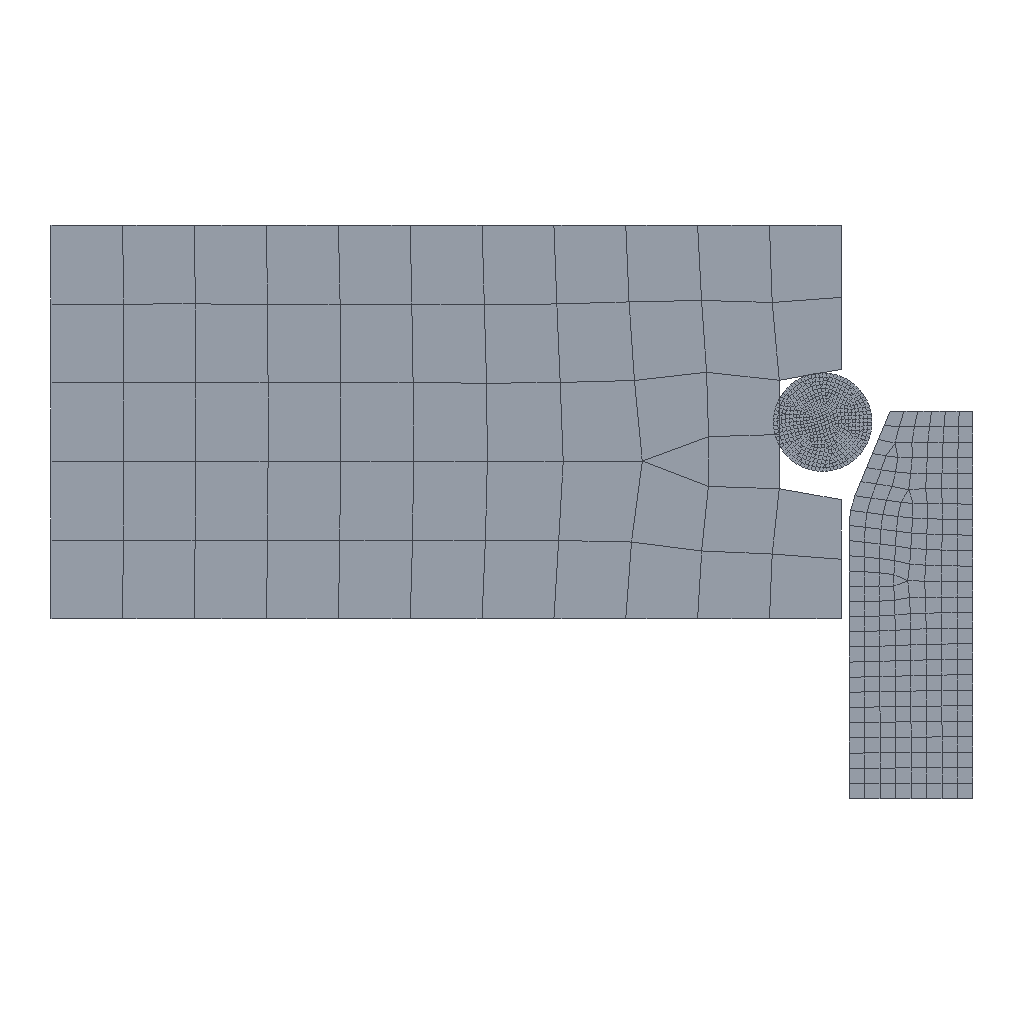Simulation study | ansys workbench
Set-up summary:
category,name,step,type,value,unit,region
solver,ansys_workbench
units,mm-N-s-tonne (MPa),,stated,"/units,MPA"
analysis,LS1,,static
load_step,LS1,LS1,static,nsubst=5; time=1
load_step,LS2,LS2,static,nsubst=100; time=2
mesh,nodes,,,2717
mesh,elements,,,1054
element_type,PLANE183,,,858
element_type,CONTA172,,,196
material,oxingquan,,behaviors,"hyperelastic; tb hype,NEO"
material,Structural Steel,,E,200000,tonne s^-2 mm^-1
material,Structural Steel,,nu,0.3
material,Structural Steel,,density,7.85e-09,tonne mm^-3
material,Structural Steel,,conductivity,60.5,tonne mm s^-3 C^-1
material,Structural Steel,,specific_heat,4.34e+08,mm^2 s^-2 C^-1
material,Structural Steel,,cte,1.2e-05,C^-1
material,Structural Steel,,permeability,10000
material,Structural Steel,,resistivity,0.00017,ohm mm
bc,Fixed Supports,model,fixed,[dofs=ALL],,_FIXEDSU
bc,Constant Zero Displacement X,model,fixed,[dofs=UX],,_DISPZEROUX
bc,Set Displacements,LS1,prescribed uy,10 [dofs=UY],,_CM54UY_YP
contact,Frictional - O ring To Surface Body,,standard (frictionless/frictional),friction=0.2; element=CONTA172
contact,Frictional - O ring To bar,,standard (frictionless/frictional),friction=0.2; element=CONTA172
named_set,_FIXEDSU,,node,23
named_set,_DISPZEROUX,,node,17
named_set,_CM54UY_YP,,node,17
Ansys APDL input file, long lists of numbers shortened:
/batch
/config,noeldb,1     ! force off writing results to database
*get,_wallstrt,active,,time,wall
! ANSYS input file written by Workbench version 2025 R2
! File used for geometry attach:
/title,O_________--____ (A5)
! ****** Begin Custom Load Command Snippet ******
/COM, ACT Extensions:
/COM,     LSDYNA, 2025.2
/COM,/COM,     ANSYSMotion, 2025.2
/COM,
! ****** End   Custom Load Command Snippet ******
*DIM,_wb_ProjectScratch_dir,string,248
_wb_ProjectScratch_dir(1) = ''
/com,--- Data in consistent NMM units. See Solving Units in the help system for more information.
/units,MPA
/nopr
/wb,file,start              !  signify a WB generated input file
/prep7
! Turn off shape checking because checks already performed inside WB mesher.
! See help system for more information.
SHPP,OFF,,NOWARN
/nolist
etcon,set             ! allow ANSYS to choose best KEYOP's for 180x elements, resets any applicable keyopt to MAPDL defaults
/com,*********** Send User Defined Coordinate System(s) ***********
csys,0
/com,*********** Nodes for the whole assembly ***********
nblock,3,,2988
(1i9,3e20.9e3)
        1     4.845794036E+01    -2.341433940E+00     0.000000000E+00
! (2716 more lines like these left out)
-1
/wb,elem,start            !  set before creation of elements
/com,*********** Elements for Body 1 'O ring' ***********
et,1,183
keyo,1,3,1
MAT,1 $ TYPE,1 $ REAL,1 $ SECNUM,1 $ ESYS,0
eblock,11,COMPACT,,605
(11i9)
       80       45       59      554      554      696     1375      554     1382
! (604 more lines like these left out)
-1
secnum,1    ! reset the section ID to default
/com,*********** Elements for Body 2 'Surface Body' ***********
et,2,183
keyo,2,3,1
MAT,2 $ TYPE,2 $ REAL,2 $ SECNUM,2 $ ESYS,0
eblock,11,COMPACT,,56
(11i9)
      650     1926     1927     1914     1914     2045     2046     1914     2047
! (55 more lines like these left out)
-1
secnum,1    ! reset the section ID to default
/com,*********** Elements for Body 3 'bar' ***********
et,3,183
keyo,3,3,1
MAT,3 $ TYPE,3 $ REAL,3 $ SECNUM,3 $ ESYS,0
eblock,11,COMPACT,,197
(11i9)
      723     2201     2203     2204     2204     2555     2557     2204     2558
! (196 more lines like these left out)
-1
secnum,1    ! reset the section ID to default
/wb,elem,end               !  done creating elements
toffst,273.15,      ! Temperature offset from absolute zero
/com,*********** Set Reference Temperature ***********
tref,22.
/wb,mat,start              !  starting to send materials
/com,*********** Send Materials ***********
TB,HYPE,1,1,1,NEO
TBDATA,1,20,0.015
Temperature = 'TEMP' ! Temperature
MP,DENS,2,7.85e-09,	! tonne mm^-3
MP,ALPX,2,1.2e-05,	! C^-1
MP,C,2,434000000,	! mm^2 s^-2 C^-1
MP,KXX,2,60.5,	! tonne mm s^-3 C^-1
MP,RSVX,2,0.00017,	! ohm mm
MP,EX,2,200000,	! tonne s^-2 mm^-1
MP,NUXY,2,0.3,
MP,MURX,2,10000,
Temperature = 'TEMP' ! Temperature
MP,DENS,3,7.85e-09,	! tonne mm^-3
MP,ALPX,3,1.2e-05,	! C^-1
MP,C,3,434000000,	! mm^2 s^-2 C^-1
MP,KXX,3,60.5,	! tonne mm s^-3 C^-1
MP,RSVX,3,0.00017,	! ohm mm
MP,EX,3,200000,	! tonne s^-2 mm^-1
MP,NUXY,3,0.3,
MP,MURX,3,10000,
/wb,mat,end                !  done sending materials
/com,*********** Send Sheet Properties ***********
!************************* Model Summary ********************
!O ring,	oxingquan,	matid,	1
!Surface Body,	ç»æé¢,	matid,	2
!bar,	ç»æé¢,	matid,	3
!************************* End Model Summary ********************
! get the diagonal of the bounding box. Needed later for other things
*get,_xmin,node,,mnloc,x
*get,_ymin,node,,mnloc,y
*get,_zmin,node,,mnloc,z
*get,_xmax,node,,mxloc,x
*get,_ymax,node,,mxloc,y
*get,_zmax,node,,mxloc,z
_ASMDIAG=(_xmax-_xmin)*(_xmax-_xmin)+(_ymax-_ymin)*(_ymax-_ymin)+(_zmax-_zmin)*(_zmax-_zmin)
_ASMDIAG=SQRT(_ASMDIAG)
/wb,contact,start          !  starting to send contact
/com,*********** Create Contact "Ä¦²ÁµÄ - O ring Î»ÓÚ Surface Body" ***********
/com,            Real Constant Set For Above Contact Is 5 & 4
*set,tid,5
*set,cid,4
r,tid
r,cid
et,tid,169
et,cid,172
MAT,4 $ TYPE,4 $ REAL,4 $ SECNUM,4 $ ESYS,0
eblock,11,COMPACT,,80
(11i9)
      859        8        9      642
! (79 more lines like these left out)
-1
secnum,1    ! reset the section ID to default
MAT,5 $ TYPE,5 $ REAL,4 $ SECNUM,5 $ ESYS,0
eblock,11,COMPACT,,4
(11i9)
      939     1887     1888     1977
      940     1888     1928     2049
      941     1928     1892     2054
      942     1892     1889     1983
-1
secnum,1    ! reset the section ID to default
keyo,cid,10,0              ! adjust contact stiffness each NR iteration (from Program Controlled setting)
keyo,cid,12,0              ! standard contact
mp,mu,cid,0.2       ! unitless
keyo,cid,2,0               ! augmented Lagrange (from Program Controlled setting)
keyo,cid,4,0               ! on Gauss point (from Program Controlled setting)
keyo,cid,9,2               ! use real geometry with ramped effects
keyo,cid,7,0               ! No Prediction
rmod,cid,3,1.       ! FKN
rmod,cid,5,0.       ! ICONT
rmod,cid,6,-2.      ! PINB
rmod,cid,10,0.      ! CNOF
rmod,cid,12,0.      ! FKT
rmod,cid,36,33      ! WB DSID
/com,*********** Create Contact "Ä¦²ÁµÄ - O ring Î»ÓÚ bar" ***********
/com,            Real Constant Set For Above Contact Is 7 & 6
*set,tid,7
*set,cid,6
r,tid
r,cid
et,tid,169
et,cid,172
MAT,6 $ TYPE,6 $ REAL,6 $ SECNUM,6 $ ESYS,0
eblock,11,COMPACT,,80
(11i9)
      943        8        9      642
! (79 more lines like these left out)
-1
secnum,1    ! reset the section ID to default
MAT,7 $ TYPE,7 $ REAL,6 $ SECNUM,7 $ ESYS,0
eblock,11,COMPACT,,32
(11i9)
     1023     2066     2291     2302
! (31 more lines like these left out)
-1
secnum,1    ! reset the section ID to default
keyo,cid,10,0              ! adjust contact stiffness each NR iteration (from Program Controlled setting)
keyo,cid,12,0              ! standard contact
mp,mu,cid,0.2       ! unitless
keyo,cid,2,0               ! augmented Lagrange (from Program Controlled setting)
keyo,cid,4,0               ! on Gauss point (from Program Controlled setting)
keyo,cid,9,2               ! use real geometry with ramped effects
keyo,cid,7,0               ! No Prediction
rmod,cid,3,1.       ! FKN
rmod,cid,5,0.       ! ICONT
rmod,cid,6,-2.      ! PINB
rmod,cid,10,0.      ! CNOF
rmod,cid,12,0.      ! FKT
rmod,cid,36,41      ! WB DSID
nsel,all
esel,all
/wb,contact,end            !  done creating contacts
/golist
/wb,load,start             !  starting to send loads
/com,*********** Fixed Supports ***********
CMBLOCK,_FIXEDSU,NODE,       23
(8i10)
      1867      1870      1872      1874      1876      1878      1880      1882
      1884      1886      1929      1930      1950      1953      1956      1959
      1962      1965      1968      1971      1974      1975      2060
cmsel,s,_FIXEDSU
d,all,all
nsel,all
/com,******* Constant Zero Displacement X *******
CMBLOCK,_DISPZEROUX,NODE,       17
(8i10)
      2087      2094      2101      2107      2114      2121      2128      2136
      2141      2359      2372      2384      2396      2408      2421      2432
      2440
cmsel,s,_DISPZEROUX
d,all,ux,0
nsel,all
/com,*********** Create Displacement Tables and Functions ******
*DIM,_loadvari54yp,TABLE,3,1,1,TIME, , , 0
! Time values
*TAXIS,_loadvari54yp(1),1,0.,1.,2.
! Load values
_loadvari54yp(1,1,1) = 0.
_loadvari54yp(2,1,1) = 0.
_loadvari54yp(3,1,1) = 10.
*DIM,_loadvari54yn,TABLE,3,1,1,TIME, , , 0
! Time values
*TAXIS,_loadvari54yn(1),1,0.,1.,2.
! Load values
_loadvari54yn(1,1,1) = 0.
_loadvari54yn(2,1,1) = 0.
_loadvari54yn(3,1,1) = -10.
/gst,on,on
fini
*get,_numnode,node,0,count
*get,_numelem,elem,0,count
*get, _MAXELEMNUM, elem, 0, NUM, MAX
*get, _MAXNODENUM, node, 0, NUM, MAX
*get, _MAXELEMTYPE, etyp, 0, NUM, MAX
*get, _MAXREALCONST, rcon, 0, NUM, MAX
/go
/wb,load,end               !  done creating loads
/com,--- Number of total nodes = %_numnode%
/com,--- Number of contact elements = 196
/com,--- Number of spring elements = 0
/com,--- Number of bearing elements = 0
/com,--- Number of solid elements = 858
/com,--- Number of condensed parts = 0
/com,--- Number of total elements = %_numelem%
*get,_wallbsol,active,,time,wall
/com,****************************************************************************
/com,*************************    SOLUTION       ********************************
/com,****************************************************************************
/solu
antype,0                   ! static analysis
nlgeom,on                  ! Turn on Large Deformation Effects
_thickRatio=  0     ! Ratio of thick parts in the model
eqsl,sparse,,,,,1
nropt,unsym                ! Use full Newton-Raphson with unsymmetric matrices
cntr,print,1               ! print out contact info and also make no initial contact an error
cncheck,dmp		!	Enable program controlled contact splitting for distributed memory parallel run
dmpoption,emat,no             ! Don't combine emat file for DANSYS
dmpoption,esav,no             ! Don't combine esav file for DANSYS
nldiag,cont,iter           ! print out contact info each equilibrium iteration
rescontrol,define,last,last,,dele	   ! Program Controlled
/com,****************************************************
/com,******************* SOLVE FOR LS 1 OF 2 ****************
/com,*** Set Displacements ***
CMBLOCK,_CM54UY_YP,NODE,       17
(8i10)
      2087      2094      2101      2107      2114      2121      2128      2136
      2141      2359      2372      2384      2396      2408      2421      2432
      2440
cmsel,s,_CM54UY_YP
d,all,uy,%_loadvari54yp%
nsel,all
/com,*** Component For All Non-Zero UY Displacements ***
cmsel,s,_CM54uy_yp
cm,_DISPNONZEROUY,NODE
nsel,all
/nopr
/gopr
autots,on                   ! User turned on automatic time stepping
nsub,5,10,3,OFF
time,1.
outres,erase
outres,all,none
outres,nsol,all,
outres,rsol,all
outres,eangl,all
outres,etmp,all
outres,veng,all
outres,strs,all,
outres,epel,all,
outres,eppl,all,
outres,cont,all,
! *********** WB SOLVE COMMAND ***********
! check interactive state
*get,ANSINTER_,active,,int
*if,ANSINTER_,ne,0,then
/eof
*endif
solve
/com *************** Write FE CONNECTORS *********
CEWRITE,file,ce,,INTE
/com,****************************************************
/com,*************** FINISHED SOLVE FOR LS 1 *************
/com,****************************************************
/com,******************* SOLVE FOR LS 2 OF 2 ****************
/com,*** Set Displacements ***
/nopr
/gopr
autots,on                   ! User turned on automatic time stepping
nsub,100,1000,100,OFF
time,2.
outres,erase
outres,all,none
outres,nsol,all,
outres,rsol,all
outres,eangl,all
outres,etmp,all
outres,veng,all
outres,strs,all,
outres,epel,all,
outres,eppl,all,
outres,cont,all,
solve
/com,****************************************************
/com,*************** FINISHED SOLVE FOR LS 2 *************
*get,_wallasol,active,,time,wall
/nopr
*get,_numnode,node,0,count
*get,_numelem,elem,0,count
*get, _MAXELEMNUM, elem, 0, NUM, MAX
*get, _MAXNODENUM, node, 0, NUM, MAX,,,INTERNAL
*get, _MAXELEMTYPE, etyp, 0, NUM, MAX
*get, _MAXREALCONST, rcon, 0, NUM, MAX
*get,_NSOLTHREADS,active,0,ntfs
*get,_NSOLPROCESSES,active,0,npfs
/gopr
/post1
xmlo,ENCODING,ISO-8859-1
xmlo,parm
/xml,parm,xml
fini
/gopr
*get,_walldone,active,,time,wall
_preptime=(_wallbsol-_wallstrt)*3600
_solvtime=(_wallasol-_wallbsol)*3600
_posttime=(_walldone-_wallasol)*3600
_totaltim=(_walldone-_wallstrt)*3600
*get,_dlbratio,active,0,solu,dlbr
*get,_combtime,active,0,solu,comb
*get,_ssmode,active,0,solu,ssmm
*get,_ndofs,active,0,solu,ndof
*get,_sol_end_time,active,0,set,time
*if,_sol_end_time,eq,2.,then
/fclean				!clean distributed files
*endif
/com,--- Total number of nodes = %_numnode%
/com,--- Total number of elements = %_numelem%
/com,--- Element load balance ratio = %_dlbratio%
/com,--- Time to combine distributed files = %_combtime%
/com,--- Sparse memory mode = %_ssmode%
/com,--- Number of DOF = %_ndofs%
/wb,file,end               ! done with WB generated input
Results summary:
result,analyses[0].index,,,1
result,analyses[0].system,,,SYS
result,analyses[0].deck,,,deck.dat
result,analyses[0].solve_status,,,completed
result,analyses[0].analysis_type,,,static
result,analyses[0].physics,,,mechanical
result,analyses[0].unit_system,,,"NMM: mm, ton, N, s, mV, mA, degC"
result,analyses[0].n_sets,,,104
result,analyses[0].load_steps[0].set,set=4,,4
result,analyses[0].load_steps[0].time_or_freq,set=4,,1
result,analyses[0].load_steps[0].max_displacement_magnitude,set=4,,0.3729
result,analyses[0].load_steps[0].max_von_mises_nodal,set=4,,0.6788
result,analyses[0].load_steps[0].reaction_force_sum_xyz[1],set=4,,36.038
result,analyses[0].load_steps[0].reaction_force_sum_xyz[2],set=4,,5.05693e-11
result,analyses[0].load_steps[0].reaction_force_sum_xyz[3],set=4,,0
result,analyses[0].load_steps[1].set,set=104,,104
result,analyses[0].load_steps[1].time_or_freq,set=104,,2
result,analyses[0].load_steps[1].max_displacement_magnitude,set=104,,10.002
result,analyses[0].load_steps[1].max_von_mises_nodal,set=104,,72.129
result,analyses[0].load_steps[1].reaction_force_sum_xyz[1],set=104,,-6218.73
result,analyses[0].load_steps[1].reaction_force_sum_xyz[2],set=104,,0.0003786
result,analyses[0].load_steps[1].reaction_force_sum_xyz[3],set=104,,0
result,geometry_export[0][0],,,.step
result,geometry_export[0][1],,,ok
result,geometry_export[0][2],,,3